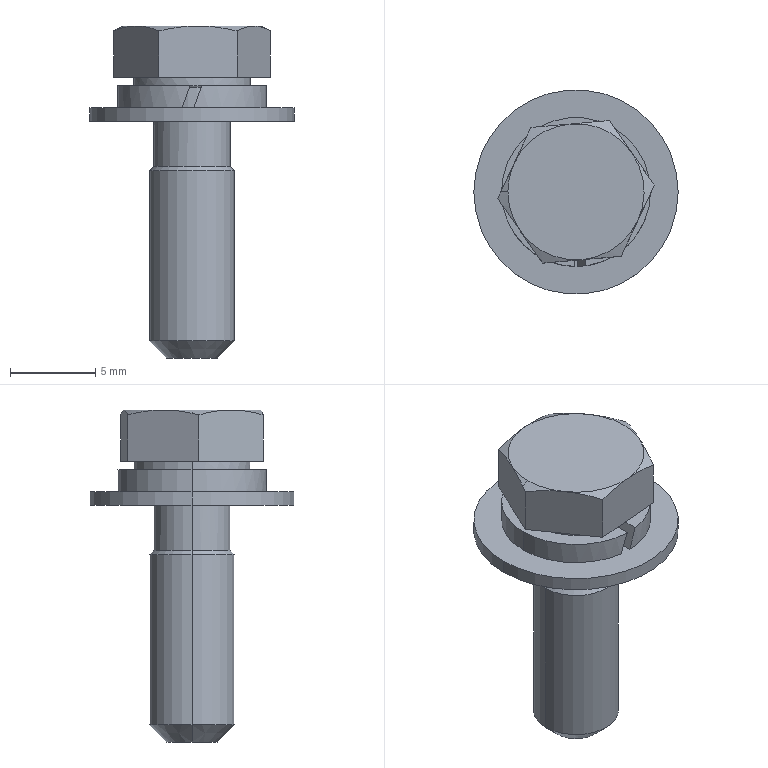Part | NX | features BREP 1 | 1 solid | 41 faces | box 12 x 12 x 19.5 mm | volume 603.235 mm3 | plane 15 | cylinder 13 | cone 11 | torus 2 | commonest cylinder face diameters 8.75 x3 4.5 x2 4.75 x2 5 x2 6.88 x2 12 x2
STEP:
#1=CARTESIAN_POINT('',(-90.692,-391.421,-6.817));
#2=VERTEX_POINT('',#1);
#3=CARTESIAN_POINT('',(-90.417,-392.5,-6.817));
#4=VERTEX_POINT('',#3);
#5=CARTESIAN_POINT('',(-92.667,-392.5,-6.817));
#6=DIRECTION('',(0.,0.,-1.));
#7=DIRECTION('',(-0.8776,-0.4794,0.));
#8=AXIS2_PLACEMENT_3D('',#5,#6,#7);
#9=CIRCLE('',#8,2.25);
#10=EDGE_CURVE('',#2,#4,#9,.T.);
#11=ORIENTED_EDGE('',*,*,#10,.F.);
#12=CARTESIAN_POINT('',(-90.604,-391.373,-6.717));
#13=VERTEX_POINT('',#12);
#14=CARTESIAN_POINT('',(-90.604,-391.373,-6.817));
#15=DIRECTION('',(-0.4794,0.8776,0.));
#16=DIRECTION('',(0.8776,0.4794,0.));
#17=AXIS2_PLACEMENT_3D('',#14,#15,#16);
#18=CIRCLE('',#17,0.1);
#19=EDGE_CURVE('',#13,#2,#18,.F.);
#20=ORIENTED_EDGE('',*,*,#19,.F.);
#21=CARTESIAN_POINT('',(-92.667,-394.85,-6.717));
#22=VERTEX_POINT('',#21);
#23=CARTESIAN_POINT('',(-90.604,-391.373,-6.717));
#24=CARTESIAN_POINT('',(-89.645,-393.129,-6.717));
#25=CARTESIAN_POINT('',(-90.666,-394.85,-6.717));
#26=CARTESIAN_POINT('',(-92.667,-394.85,-6.717));
#27=(BOUNDED_CURVE()B_SPLINE_CURVE(3,(#23,#24,#25,#26),.UNSPECIFIED.,.F.,.F.)B_SPLINE_CURVE_WITH_KNOTS((4,4),(0.,1.),.PIECEWISE_BEZIER_KNOTS.)CURVE()GEOMETRIC_REPRESENTATION_ITEM()RATIONAL_B_SPLINE_CURVE((1.,0.6735,0.6735,1.))REPRESENTATION_ITEM(''));
#28=EDGE_CURVE('',#13,#22,#27,.T.);
#29=ORIENTED_EDGE('',*,*,#28,.T.);
#30=CARTESIAN_POINT('',(-94.729,-393.627,-6.717));
#31=VERTEX_POINT('',#30);
#32=CARTESIAN_POINT('',(-92.667,-394.85,-6.717));
#33=CARTESIAN_POINT('',(-93.548,-394.85,-6.717));
#34=CARTESIAN_POINT('',(-94.306,-394.4,-6.717));
#35=CARTESIAN_POINT('',(-94.729,-393.627,-6.717));
#36=(BOUNDED_CURVE()B_SPLINE_CURVE(3,(#32,#33,#34,#35),.UNSPECIFIED.,.F.,.F.)B_SPLINE_CURVE_WITH_KNOTS((4,4),(0.,1.),.PIECEWISE_BEZIER_KNOTS.)CURVE()GEOMETRIC_REPRESENTATION_ITEM()RATIONAL_B_SPLINE_CURVE((1.,0.9067,0.9067,1.))REPRESENTATION_ITEM(''));
#37=EDGE_CURVE('',#22,#31,#36,.T.);
#38=ORIENTED_EDGE('',*,*,#37,.T.);
#39=CARTESIAN_POINT('',(-94.641,-393.579,-6.817));
#40=VERTEX_POINT('',#39);
#41=CARTESIAN_POINT('',(-94.729,-393.627,-6.817));
#42=DIRECTION('',(0.4794,-0.8776,0.));
#43=DIRECTION('',(-0.8776,-0.4794,0.));
#44=AXIS2_PLACEMENT_3D('',#41,#42,#43);
#45=CIRCLE('',#44,0.1);
#46=EDGE_CURVE('',#31,#40,#45,.F.);
#47=ORIENTED_EDGE('',*,*,#46,.T.);
#48=CARTESIAN_POINT('',(-92.667,-392.5,-6.817));
#49=DIRECTION('',(0.,0.,-1.));
#50=DIRECTION('',(-0.8776,-0.4794,0.));
#51=AXIS2_PLACEMENT_3D('',#48,#49,#50);
#52=CIRCLE('',#51,2.25);
#53=EDGE_CURVE('',#4,#40,#52,.T.);
#54=ORIENTED_EDGE('',*,*,#53,.F.);
#55=EDGE_LOOP('',(#11,#20,#29,#38,#47,#54));
#56=FACE_BOUND('',#55,.T.);
#57=CARTESIAN_POINT('',(-92.667,-392.5,-6.817));
#58=DIRECTION('',(0.,0.,1.));
#59=DIRECTION('',(1.,0.,0.));
#60=AXIS2_PLACEMENT_3D('',#57,#58,#59);
#61=TOROIDAL_SURFACE('',#60,2.35,0.1);
#62=ADVANCED_FACE('',(#56),#61,.F.);
#63=CARTESIAN_POINT('',(-90.292,-392.5,-6.717));
#64=VERTEX_POINT('',#63);
#65=CARTESIAN_POINT('',(-92.084,-394.802,-6.717));
#66=VERTEX_POINT('',#65);
#67=CARTESIAN_POINT('',(-92.667,-392.5,-6.717));
#68=DIRECTION('',(0.,0.,-1.));
#69=DIRECTION('',(-1.,0.,0.));
#70=AXIS2_PLACEMENT_3D('',#67,#68,#69);
#71=CIRCLE('',#70,2.375);
#72=EDGE_CURVE('',#64,#66,#71,.T.);
#73=ORIENTED_EDGE('',*,*,#72,.F.);
#74=CARTESIAN_POINT('',(-90.292,-392.5,-8.817));
#75=VERTEX_POINT('',#74);
#76=CARTESIAN_POINT('',(-90.292,-392.5,-7.367));
#77=DIRECTION('',(0.,0.,-1.));
#78=VECTOR('',#77,1000.);
#79=LINE('',#76,#78);
#80=EDGE_CURVE('',#75,#64,#79,.F.);
#81=ORIENTED_EDGE('',*,*,#80,.F.);
#82=CARTESIAN_POINT('',(-95.042,-392.5,-8.817));
#83=VERTEX_POINT('',#82);
#84=CARTESIAN_POINT('',(-92.667,-392.5,-8.817));
#85=DIRECTION('',(0.,0.,1.));
#86=DIRECTION('',(-1.,0.,0.));
#87=AXIS2_PLACEMENT_3D('',#84,#85,#86);
#88=CIRCLE('',#87,2.375);
#89=EDGE_CURVE('',#83,#75,#88,.T.);
#90=ORIENTED_EDGE('',*,*,#89,.F.);
#91=CARTESIAN_POINT('',(-95.042,-392.5,-6.717));
#92=VERTEX_POINT('',#91);
#93=CARTESIAN_POINT('',(-95.042,-392.5,-7.367));
#94=DIRECTION('',(0.,0.,-1.));
#95=VECTOR('',#94,1000.);
#96=LINE('',#93,#95);
#97=EDGE_CURVE('',#83,#92,#96,.F.);
#98=ORIENTED_EDGE('',*,*,#97,.T.);
#99=CARTESIAN_POINT('',(-92.776,-394.872,-6.717));
#100=VERTEX_POINT('',#99);
#101=CARTESIAN_POINT('',(-92.667,-392.5,-6.717));
#102=DIRECTION('',(0.,0.,-1.));
#103=DIRECTION('',(-1.,0.,0.));
#104=AXIS2_PLACEMENT_3D('',#101,#102,#103);
#105=CIRCLE('',#104,2.375);
#106=EDGE_CURVE('',#100,#92,#105,.T.);
#107=ORIENTED_EDGE('',*,*,#106,.F.);
#108=CARTESIAN_POINT('',(-93.249,-394.802,-8.017));
#109=VERTEX_POINT('',#108);
#110=CARTESIAN_POINT('',(-93.249,-394.802,-8.017));
#111=CARTESIAN_POINT('',(-93.094,-394.842,-7.591));
#112=CARTESIAN_POINT('',(-92.936,-394.865,-7.156));
#113=CARTESIAN_POINT('',(-92.776,-394.872,-6.717));
#114=(BOUNDED_CURVE()B_SPLINE_CURVE(3,(#110,#111,#112,#113),.UNSPECIFIED.,.F.,.F.)B_SPLINE_CURVE_WITH_KNOTS((4,4),(0.,1.),.PIECEWISE_BEZIER_KNOTS.)CURVE()GEOMETRIC_REPRESENTATION_ITEM()RATIONAL_B_SPLINE_CURVE((1.,0.9966,0.9966,1.))REPRESENTATION_ITEM(''));
#115=EDGE_CURVE('',#109,#100,#114,.T.);
#116=ORIENTED_EDGE('',*,*,#115,.F.);
#117=CARTESIAN_POINT('',(-92.557,-394.872,-8.017));
#118=VERTEX_POINT('',#117);
#119=CARTESIAN_POINT('',(-92.667,-392.5,-8.017));
#120=DIRECTION('',(0.,0.,1.));
#121=DIRECTION('',(-1.,0.,0.));
#122=AXIS2_PLACEMENT_3D('',#119,#120,#121);
#123=CIRCLE('',#122,2.375);
#124=EDGE_CURVE('',#109,#118,#123,.T.);
#125=ORIENTED_EDGE('',*,*,#124,.T.);
#126=CARTESIAN_POINT('',(-92.084,-394.802,-6.717));
#127=CARTESIAN_POINT('',(-92.239,-394.842,-7.143));
#128=CARTESIAN_POINT('',(-92.398,-394.865,-7.578));
#129=CARTESIAN_POINT('',(-92.557,-394.872,-8.017));
#130=(BOUNDED_CURVE()B_SPLINE_CURVE(3,(#126,#127,#128,#129),.UNSPECIFIED.,.F.,.F.)B_SPLINE_CURVE_WITH_KNOTS((4,4),(0.,1.),.PIECEWISE_BEZIER_KNOTS.)CURVE()GEOMETRIC_REPRESENTATION_ITEM()RATIONAL_B_SPLINE_CURVE((1.,0.9966,0.9966,1.))REPRESENTATION_ITEM(''));
#131=EDGE_CURVE('',#66,#118,#130,.T.);
#132=ORIENTED_EDGE('',*,*,#131,.F.);
#133=EDGE_LOOP('',(#73,#81,#90,#98,#107,#116,#125,#132));
#134=FACE_BOUND('',#133,.T.);
#135=CARTESIAN_POINT('',(-92.667,-392.5,-7.367));
#136=DIRECTION('',(0.,0.,-1.));
#137=DIRECTION('',(1.,0.,0.));
#138=AXIS2_PLACEMENT_3D('',#135,#136,#137);
#139=CYLINDRICAL_SURFACE('',#138,2.375);
#140=ADVANCED_FACE('',(#134),#139,.F.);
#141=CARTESIAN_POINT('',(-98.667,-392.5,-8.017));
#142=VERTEX_POINT('',#141);
#143=CARTESIAN_POINT('',(-86.667,-392.5,-8.017));
#144=VERTEX_POINT('',#143);
#145=CARTESIAN_POINT('',(-92.667,-392.5,-8.017));
#146=DIRECTION('',(0.,0.,-1.));
#147=DIRECTION('',(-1.,0.,0.));
#148=AXIS2_PLACEMENT_3D('',#145,#146,#147);
#149=CIRCLE('',#148,6.);
#150=EDGE_CURVE('',#142,#144,#149,.T.);
#151=ORIENTED_EDGE('',*,*,#150,.T.);
#152=CARTESIAN_POINT('',(-86.667,-392.5,-8.817));
#153=VERTEX_POINT('',#152);
#154=CARTESIAN_POINT('',(-86.667,-392.5,-8.517));
#155=DIRECTION('',(0.,0.,-1.));
#156=VECTOR('',#155,1000.);
#157=LINE('',#154,#156);
#158=EDGE_CURVE('',#153,#144,#157,.F.);
#159=ORIENTED_EDGE('',*,*,#158,.F.);
#160=CARTESIAN_POINT('',(-98.667,-392.5,-8.817));
#161=VERTEX_POINT('',#160);
#162=CARTESIAN_POINT('',(-92.667,-392.5,-8.817));
#163=DIRECTION('',(0.,0.,-1.));
#164=DIRECTION('',(-1.,0.,0.));
#165=AXIS2_PLACEMENT_3D('',#162,#163,#164);
#166=CIRCLE('',#165,6.);
#167=EDGE_CURVE('',#161,#153,#166,.T.);
#168=ORIENTED_EDGE('',*,*,#167,.F.);
#169=CARTESIAN_POINT('',(-98.667,-392.5,-8.517));
#170=DIRECTION('',(0.,0.,-1.));
#171=VECTOR('',#170,1000.);
#172=LINE('',#169,#171);
#173=EDGE_CURVE('',#161,#142,#172,.F.);
#174=ORIENTED_EDGE('',*,*,#173,.T.);
#175=EDGE_LOOP('',(#151,#159,#168,#174));
#176=FACE_BOUND('',#175,.T.);
#177=CARTESIAN_POINT('',(-92.667,-392.5,-8.517));
#178=DIRECTION('',(0.,0.,-1.));
#179=DIRECTION('',(1.,0.,0.));
#180=AXIS2_PLACEMENT_3D('',#177,#178,#179);
#181=CYLINDRICAL_SURFACE('',#180,6.);
#182=ADVANCED_FACE('',(#176),#181,.T.);
#183=CARTESIAN_POINT('',(-97.042,-392.5,-6.717));
#184=VERTEX_POINT('',#183);
#185=CARTESIAN_POINT('',(-88.292,-392.5,-6.717));
#186=VERTEX_POINT('',#185);
#187=CARTESIAN_POINT('',(-92.667,-392.5,-6.717));
#188=DIRECTION('',(0.,0.,-1.));
#189=DIRECTION('',(-1.,0.,0.));
#190=AXIS2_PLACEMENT_3D('',#187,#188,#189);
#191=CIRCLE('',#190,4.375);
#192=EDGE_CURVE('',#184,#186,#191,.T.);
#193=ORIENTED_EDGE('',*,*,#192,.T.);
#194=CARTESIAN_POINT('',(-88.292,-392.5,-8.017));
#195=VERTEX_POINT('',#194);
#196=CARTESIAN_POINT('',(-88.292,-392.5,-7.367));
#197=DIRECTION('',(0.,0.,-1.));
#198=VECTOR('',#197,1000.);
#199=LINE('',#196,#198);
#200=EDGE_CURVE('',#186,#195,#199,.T.);
#201=ORIENTED_EDGE('',*,*,#200,.T.);
#202=CARTESIAN_POINT('',(-97.042,-392.5,-8.017));
#203=VERTEX_POINT('',#202);
#204=CARTESIAN_POINT('',(-92.667,-392.5,-8.017));
#205=DIRECTION('',(0.,0.,1.));
#206=DIRECTION('',(-1.,0.,0.));
#207=AXIS2_PLACEMENT_3D('',#204,#205,#206);
#208=CIRCLE('',#207,4.375);
#209=EDGE_CURVE('',#195,#203,#208,.T.);
#210=ORIENTED_EDGE('',*,*,#209,.T.);
#211=CARTESIAN_POINT('',(-97.042,-392.5,-7.367));
#212=DIRECTION('',(0.,0.,-1.));
#213=VECTOR('',#212,1000.);
#214=LINE('',#211,#213);
#215=EDGE_CURVE('',#184,#203,#214,.T.);
#216=ORIENTED_EDGE('',*,*,#215,.F.);
#217=EDGE_LOOP('',(#193,#201,#210,#216));
#218=FACE_BOUND('',#217,.T.);
#219=CARTESIAN_POINT('',(-92.667,-392.5,-7.367));
#220=DIRECTION('',(0.,0.,-1.));
#221=DIRECTION('',(1.,0.,0.));
#222=AXIS2_PLACEMENT_3D('',#219,#220,#221);
#223=CYLINDRICAL_SURFACE('',#222,4.375);
#224=ADVANCED_FACE('',(#218),#223,.T.);
#225=CARTESIAN_POINT('',(-92.776,-396.874,-6.717));
#226=VERTEX_POINT('',#225);
#227=CARTESIAN_POINT('',(-92.667,-392.5,-6.717));
#228=DIRECTION('',(0.,0.,-1.));
#229=DIRECTION('',(-1.,0.,0.));
#230=AXIS2_PLACEMENT_3D('',#227,#228,#229);
#231=CIRCLE('',#230,4.375);
#232=EDGE_CURVE('',#226,#184,#231,.T.);
#233=ORIENTED_EDGE('',*,*,#232,.T.);
#234=ORIENTED_EDGE('',*,*,#215,.T.);
#235=CARTESIAN_POINT('',(-93.249,-396.836,-8.017));
#236=VERTEX_POINT('',#235);
#237=CARTESIAN_POINT('',(-92.667,-392.5,-8.017));
#238=DIRECTION('',(0.,0.,1.));
#239=DIRECTION('',(-1.,0.,0.));
#240=AXIS2_PLACEMENT_3D('',#237,#238,#239);
#241=CIRCLE('',#240,4.375);
#242=EDGE_CURVE('',#203,#236,#241,.T.);
#243=ORIENTED_EDGE('',*,*,#242,.T.);
#244=CARTESIAN_POINT('',(-93.249,-396.836,-8.017));
#245=CARTESIAN_POINT('',(-93.092,-396.857,-7.585));
#246=CARTESIAN_POINT('',(-92.934,-396.87,-7.152));
#247=CARTESIAN_POINT('',(-92.776,-396.874,-6.717));
#248=(BOUNDED_CURVE()B_SPLINE_CURVE(3,(#244,#245,#246,#247),.UNSPECIFIED.,.F.,.F.)B_SPLINE_CURVE_WITH_KNOTS((4,4),(0.,1.),.PIECEWISE_BEZIER_KNOTS.)CURVE()GEOMETRIC_REPRESENTATION_ITEM()RATIONAL_B_SPLINE_CURVE((1.,0.999,0.999,1.))REPRESENTATION_ITEM(''));
#249=EDGE_CURVE('',#236,#226,#248,.T.);
#250=ORIENTED_EDGE('',*,*,#249,.T.);
#251=EDGE_LOOP('',(#233,#234,#243,#250));
#252=FACE_BOUND('',#251,.T.);
#253=CARTESIAN_POINT('',(-92.667,-392.5,-7.367));
#254=DIRECTION('',(0.,0.,-1.));
#255=DIRECTION('',(1.,0.,0.));
#256=AXIS2_PLACEMENT_3D('',#253,#254,#255);
#257=CYLINDRICAL_SURFACE('',#256,4.375);
#258=ADVANCED_FACE('',(#252),#257,.T.);
#259=CARTESIAN_POINT('',(-90.417,-392.5,-11.468));
#260=VERTEX_POINT('',#259);
#261=CARTESIAN_POINT('',(-94.917,-392.5,-11.468));
#262=VERTEX_POINT('',#261);
#263=CARTESIAN_POINT('',(-92.667,-392.5,-11.468));
#264=DIRECTION('',(0.,0.,1.));
#265=DIRECTION('',(1.,0.,0.));
#266=AXIS2_PLACEMENT_3D('',#263,#264,#265);
#267=CIRCLE('',#266,2.25);
#268=EDGE_CURVE('',#260,#262,#267,.T.);
#269=ORIENTED_EDGE('',*,*,#268,.T.);
#270=CARTESIAN_POINT('',(-94.917,-392.5,-6.817));
#271=VERTEX_POINT('',#270);
#272=CARTESIAN_POINT('',(-94.917,-392.5,-12.967));
#273=DIRECTION('',(0.,0.,1.));
#274=VECTOR('',#273,1000.);
#275=LINE('',#272,#274);
#276=EDGE_CURVE('',#262,#271,#275,.T.);
#277=ORIENTED_EDGE('',*,*,#276,.T.);
#278=CARTESIAN_POINT('',(-92.667,-392.5,-6.817));
#279=DIRECTION('',(0.,0.,-1.));
#280=DIRECTION('',(-0.8776,-0.4794,0.));
#281=AXIS2_PLACEMENT_3D('',#278,#279,#280);
#282=CIRCLE('',#281,2.25);
#283=EDGE_CURVE('',#271,#2,#282,.T.);
#284=ORIENTED_EDGE('',*,*,#283,.T.);
#285=ORIENTED_EDGE('',*,*,#10,.T.);
#286=CARTESIAN_POINT('',(-90.417,-392.5,-12.967));
#287=DIRECTION('',(0.,0.,1.));
#288=VECTOR('',#287,1000.);
#289=LINE('',#286,#288);
#290=EDGE_CURVE('',#260,#4,#289,.T.);
#291=ORIENTED_EDGE('',*,*,#290,.F.);
#292=EDGE_LOOP('',(#269,#277,#284,#285,#291));
#293=FACE_BOUND('',#292,.T.);
#294=CARTESIAN_POINT('',(-92.667,-392.5,-12.967));
#295=DIRECTION('',(0.,0.,1.));
#296=DIRECTION('',(-1.,0.,0.));
#297=AXIS2_PLACEMENT_3D('',#294,#295,#296);
#298=CYLINDRICAL_SURFACE('',#297,2.25);
#299=ADVANCED_FACE('',(#293),#298,.T.);
#300=ORIENTED_EDGE('',*,*,#268,.F.);
#301=CARTESIAN_POINT('',(-90.167,-392.5,-11.718));
#302=VERTEX_POINT('',#301);
#303=CARTESIAN_POINT('',(-90.167,-392.5,-11.718));
#304=DIRECTION('',(0.7071,0.,-0.7071));
#305=VECTOR('',#304,1000.);
#306=LINE('',#303,#305);
#307=EDGE_CURVE('',#302,#260,#306,.F.);
#308=ORIENTED_EDGE('',*,*,#307,.F.);
#309=CARTESIAN_POINT('',(-95.167,-392.5,-11.718));
#310=VERTEX_POINT('',#309);
#311=CARTESIAN_POINT('',(-92.667,-392.5,-11.718));
#312=DIRECTION('',(0.,0.,1.));
#313=DIRECTION('',(0.8776,0.4794,0.));
#314=AXIS2_PLACEMENT_3D('',#311,#312,#313);
#315=CIRCLE('',#314,2.5);
#316=EDGE_CURVE('',#302,#310,#315,.T.);
#317=ORIENTED_EDGE('',*,*,#316,.T.);
#318=CARTESIAN_POINT('',(-95.167,-392.5,-11.718));
#319=DIRECTION('',(-0.7071,0.,-0.7071));
#320=VECTOR('',#319,1000.);
#321=LINE('',#318,#320);
#322=EDGE_CURVE('',#310,#262,#321,.F.);
#323=ORIENTED_EDGE('',*,*,#322,.T.);
#324=EDGE_LOOP('',(#300,#308,#317,#323));
#325=FACE_BOUND('',#324,.T.);
#326=CARTESIAN_POINT('',(-92.667,-392.5,-11.718));
#327=DIRECTION('',(0.,0.,-1.));
#328=DIRECTION('',(1.,0.,0.));
#329=AXIS2_PLACEMENT_3D('',#326,#327,#328);
#330=CONICAL_SURFACE('',#329,2.5,0.7854);
#331=ADVANCED_FACE('',(#325),#330,.T.);
#332=CARTESIAN_POINT('',(-96.107,-392.5,-6.717));
#333=VERTEX_POINT('',#332);
#334=CARTESIAN_POINT('',(-89.227,-392.5,-6.717));
#335=VERTEX_POINT('',#334);
#336=CARTESIAN_POINT('',(-92.667,-392.5,-6.717));
#337=DIRECTION('',(0.,0.,-1.));
#338=DIRECTION('',(1.,0.,0.));
#339=AXIS2_PLACEMENT_3D('',#336,#337,#338);
#340=CIRCLE('',#339,3.44);
#341=EDGE_CURVE('',#333,#335,#340,.T.);
#342=ORIENTED_EDGE('',*,*,#341,.F.);
#343=CARTESIAN_POINT('',(-96.107,-392.5,-6.217));
#344=VERTEX_POINT('',#343);
#345=CARTESIAN_POINT('',(-96.107,-392.5,-12.967));
#346=DIRECTION('',(0.,0.,1.));
#347=VECTOR('',#346,1000.);
#348=LINE('',#345,#347);
#349=EDGE_CURVE('',#333,#344,#348,.T.);
#350=ORIENTED_EDGE('',*,*,#349,.T.);
#351=CARTESIAN_POINT('',(-89.227,-392.5,-6.217));
#352=VERTEX_POINT('',#351);
#353=CARTESIAN_POINT('',(-92.667,-392.5,-6.217));
#354=DIRECTION('',(0.,0.,-1.));
#355=DIRECTION('',(1.,0.,0.));
#356=AXIS2_PLACEMENT_3D('',#353,#354,#355);
#357=CIRCLE('',#356,3.44);
#358=EDGE_CURVE('',#344,#352,#357,.T.);
#359=ORIENTED_EDGE('',*,*,#358,.T.);
#360=CARTESIAN_POINT('',(-89.227,-392.5,-12.967));
#361=DIRECTION('',(0.,0.,1.));
#362=VECTOR('',#361,1000.);
#363=LINE('',#360,#362);
#364=EDGE_CURVE('',#335,#352,#363,.T.);
#365=ORIENTED_EDGE('',*,*,#364,.F.);
#366=EDGE_LOOP('',(#342,#350,#359,#365));
#367=FACE_BOUND('',#366,.T.);
#368=CARTESIAN_POINT('',(-92.667,-392.5,-12.967));
#369=DIRECTION('',(0.,0.,1.));
#370=DIRECTION('',(-1.,0.,0.));
#371=AXIS2_PLACEMENT_3D('',#368,#369,#370);
#372=CYLINDRICAL_SURFACE('',#371,3.44);
#373=ADVANCED_FACE('',(#367),#372,.T.);
#374=CARTESIAN_POINT('',(-90.167,-392.5,-21.717));
#375=VERTEX_POINT('',#374);
#376=CARTESIAN_POINT('',(-95.167,-392.5,-21.717));
#377=VERTEX_POINT('',#376);
#378=CARTESIAN_POINT('',(-92.667,-392.5,-21.717));
#379=DIRECTION('',(0.,0.,1.));
#380=DIRECTION('',(1.,0.,0.));
#381=AXIS2_PLACEMENT_3D('',#378,#379,#380);
#382=CIRCLE('',#381,2.5);
#383=EDGE_CURVE('',#375,#377,#382,.T.);
#384=ORIENTED_EDGE('',*,*,#383,.T.);
#385=CARTESIAN_POINT('',(-95.167,-392.5,-12.967));
#386=DIRECTION('',(0.,0.,1.));
#387=VECTOR('',#386,1000.);
#388=LINE('',#385,#387);
#389=EDGE_CURVE('',#377,#310,#388,.T.);
#390=ORIENTED_EDGE('',*,*,#389,.T.);
#391=ORIENTED_EDGE('',*,*,#316,.F.);
#392=CARTESIAN_POINT('',(-90.167,-392.5,-12.967));
#393=DIRECTION('',(0.,0.,1.));
#394=VECTOR('',#393,1000.);
#395=LINE('',#392,#394);
#396=EDGE_CURVE('',#375,#302,#395,.T.);
#397=ORIENTED_EDGE('',*,*,#396,.F.);
#398=EDGE_LOOP('',(#384,#390,#391,#397));
#399=FACE_BOUND('',#398,.T.);
#400=CARTESIAN_POINT('',(-92.667,-392.5,-12.967));
#401=DIRECTION('',(0.,0.,1.));
#402=DIRECTION('',(-1.,0.,0.));
#403=AXIS2_PLACEMENT_3D('',#400,#401,#402);
#404=CYLINDRICAL_SURFACE('',#403,2.5);
#405=ADVANCED_FACE('',(#399),#404,.T.);
#406=CARTESIAN_POINT('',(-91.167,-392.5,-22.717));
#407=VERTEX_POINT('',#406);
#408=CARTESIAN_POINT('',(-94.167,-392.5,-22.717));
#409=VERTEX_POINT('',#408);
#410=CARTESIAN_POINT('',(-92.667,-392.5,-22.717));
#411=DIRECTION('',(0.,0.,1.));
#412=DIRECTION('',(1.,0.,0.));
#413=AXIS2_PLACEMENT_3D('',#410,#411,#412);
#414=CIRCLE('',#413,1.5);
#415=EDGE_CURVE('',#407,#409,#414,.T.);
#416=ORIENTED_EDGE('',*,*,#415,.T.);
#417=CARTESIAN_POINT('',(-95.167,-392.5,-21.717));
#418=DIRECTION('',(-0.7071,0.,0.7071));
#419=VECTOR('',#418,1000.);
#420=LINE('',#417,#419);
#421=EDGE_CURVE('',#409,#377,#420,.T.);
#422=ORIENTED_EDGE('',*,*,#421,.T.);
#423=ORIENTED_EDGE('',*,*,#383,.F.);
#424=CARTESIAN_POINT('',(-90.167,-392.5,-21.717));
#425=DIRECTION('',(0.7071,0.,0.7071));
#426=VECTOR('',#425,1000.);
#427=LINE('',#424,#426);
#428=EDGE_CURVE('',#407,#375,#427,.T.);
#429=ORIENTED_EDGE('',*,*,#428,.F.);
#430=EDGE_LOOP('',(#416,#422,#423,#429));
#431=FACE_BOUND('',#430,.T.);
#432=CARTESIAN_POINT('',(-92.667,-392.5,-21.717));
#433=DIRECTION('',(0.,0.,1.));
#434=DIRECTION('',(-1.,0.,0.));
#435=AXIS2_PLACEMENT_3D('',#432,#433,#434);
#436=CONICAL_SURFACE('',#435,2.5,0.7854);
#437=ADVANCED_FACE('',(#431),#436,.T.);
#438=CARTESIAN_POINT('',(-95.943,-394.794,-3.217));
#439=VERTEX_POINT('',#438);
#440=CARTESIAN_POINT('',(-96.667,-392.5,-3.217));
#441=VERTEX_POINT('',#440);
#442=CARTESIAN_POINT('',(-92.667,-392.5,-3.217));
#443=DIRECTION('',(0.,0.,-1.));
#444=DIRECTION('',(-1.,0.,0.));
#445=AXIS2_PLACEMENT_3D('',#442,#443,#444);
#446=CIRCLE('',#445,4.);
#447=EDGE_CURVE('',#439,#441,#446,.T.);
#448=ORIENTED_EDGE('',*,*,#447,.T.);
#449=CARTESIAN_POINT('',(-97.08,-392.5,-3.409));
#450=VERTEX_POINT('',#449);
#451=CARTESIAN_POINT('',(-97.289,-392.5,-3.507));
#452=DIRECTION('',(-0.9063,0.,-0.4226));
#453=VECTOR('',#452,1000.);
#454=LINE('',#451,#453);
#455=EDGE_CURVE('',#441,#450,#454,.T.);
#456=ORIENTED_EDGE('',*,*,#455,.T.);
#457=CARTESIAN_POINT('',(-97.268,-392.903,-3.505));
#458=VERTEX_POINT('',#457);
#459=CARTESIAN_POINT('',(-97.08,-392.5,-3.409));
#460=CARTESIAN_POINT('',(-97.142,-392.633,-3.438));
#461=CARTESIAN_POINT('',(-97.204,-392.767,-3.47));
#462=CARTESIAN_POINT('',(-97.268,-392.903,-3.505));
#463=B_SPLINE_CURVE_WITH_KNOTS('',3,(#459,#460,#461,#462),.UNSPECIFIED.,.F.,.F.,(4,4),(0.,1.),.PIECEWISE_BEZIER_KNOTS.);
#464=EDGE_CURVE('',#450,#458,#463,.T.);
#465=ORIENTED_EDGE('',*,*,#464,.T.);
#466=CARTESIAN_POINT('',(-97.268,-392.903,-3.505));
#467=CARTESIAN_POINT('',(-96.832,-393.525,-3.328));
#468=CARTESIAN_POINT('',(-96.392,-394.154,-3.217));
#469=CARTESIAN_POINT('',(-95.943,-394.794,-3.217));
#470=B_SPLINE_CURVE_WITH_KNOTS('',3,(#466,#467,#468,#469),.UNSPECIFIED.,.F.,.F.,(4,4),(0.,0.002327),.UNSPECIFIED.);
#471=EDGE_CURVE('',#458,#439,#470,.T.);
#472=ORIENTED_EDGE('',*,*,#471,.T.);
#473=EDGE_LOOP('',(#448,#456,#465,#472));
#474=FACE_BOUND('',#473,.T.);
#475=CARTESIAN_POINT('',(-92.667,-392.5,-3.507));
#476=DIRECTION('',(0.,0.,-1.));
#477=DIRECTION('',(1.,0.,0.));
#478=AXIS2_PLACEMENT_3D('',#475,#476,#477);
#479=CONICAL_SURFACE('',#478,4.623,1.134);
#480=ADVANCED_FACE('',(#474),#479,.T.);
#481=ORIENTED_EDGE('',*,*,#89,.T.);
#482=CARTESIAN_POINT('',(-92.667,-392.5,-8.817));
#483=DIRECTION('',(0.,0.,1.));
#484=DIRECTION('',(-1.,0.,0.));
#485=AXIS2_PLACEMENT_3D('',#482,#483,#484);
#486=CIRCLE('',#485,2.375);
#487=EDGE_CURVE('',#75,#83,#486,.T.);
#488=ORIENTED_EDGE('',*,*,#487,.T.);
#489=EDGE_LOOP('',(#481,#488));
#490=FACE_BOUND('',#489,.T.);
#491=ORIENTED_EDGE('',*,*,#167,.T.);
#492=CARTESIAN_POINT('',(-92.667,-392.5,-8.817));
#493=DIRECTION('',(0.,0.,-1.));
#494=DIRECTION('',(-1.,0.,0.));
#495=AXIS2_PLACEMENT_3D('',#492,#493,#494);
#496=CIRCLE('',#495,6.);
#497=EDGE_CURVE('',#153,#161,#496,.T.);
#498=ORIENTED_EDGE('',*,*,#497,.T.);
#499=EDGE_LOOP('',(#491,#498));
#500=FACE_BOUND('',#499,.T.);
#501=CARTESIAN_POINT('',(-92.667,-392.5,-8.817));
#502=DIRECTION('',(0.,0.,-1.));
#503=DIRECTION('',(1.,0.,0.));
#504=AXIS2_PLACEMENT_3D('',#501,#502,#503);
#505=PLANE('',#504);
#506=ADVANCED_FACE('',(#490,#500),#505,.T.);
#507=ORIENTED_EDGE('',*,*,#80,.T.);
#508=CARTESIAN_POINT('',(-92.667,-392.5,-6.717));
#509=DIRECTION('',(0.,0.,-1.));
#510=DIRECTION('',(-1.,0.,0.));
#511=AXIS2_PLACEMENT_3D('',#508,#509,#510);
#512=CIRCLE('',#511,2.375);
#513=EDGE_CURVE('',#92,#64,#512,.T.);
#514=ORIENTED_EDGE('',*,*,#513,.F.);
#515=ORIENTED_EDGE('',*,*,#97,.F.);
#516=ORIENTED_EDGE('',*,*,#487,.F.);
#517=EDGE_LOOP('',(#507,#514,#515,#516));
#518=FACE_BOUND('',#517,.T.);
#519=CARTESIAN_POINT('',(-92.667,-392.5,-7.367));
#520=DIRECTION('',(0.,0.,-1.));
#521=DIRECTION('',(1.,0.,0.));
#522=AXIS2_PLACEMENT_3D('',#519,#520,#521);
#523=CYLINDRICAL_SURFACE('',#522,2.375);
#524=ADVANCED_FACE('',(#518),#523,.F.);
#525=ORIENTED_EDGE('',*,*,#158,.T.);
#526=CARTESIAN_POINT('',(-92.667,-392.5,-8.017));
#527=DIRECTION('',(0.,0.,-1.));
#528=DIRECTION('',(-1.,0.,0.));
#529=AXIS2_PLACEMENT_3D('',#526,#527,#528);
#530=CIRCLE('',#529,6.);
#531=EDGE_CURVE('',#144,#142,#530,.T.);
#532=ORIENTED_EDGE('',*,*,#531,.T.);
#533=ORIENTED_EDGE('',*,*,#173,.F.);
#534=ORIENTED_EDGE('',*,*,#497,.F.);
#535=EDGE_LOOP('',(#525,#532,#533,#534));
#536=FACE_BOUND('',#535,.T.);
#537=CARTESIAN_POINT('',(-92.667,-392.5,-8.517));
#538=DIRECTION('',(0.,0.,-1.));
#539=DIRECTION('',(1.,0.,0.));
#540=AXIS2_PLACEMENT_3D('',#537,#538,#539);
#541=CYLINDRICAL_SURFACE('',#540,6.);
#542=ADVANCED_FACE('',(#536),#541,.T.);
#543=ORIENTED_EDGE('',*,*,#28,.F.);
#544=CARTESIAN_POINT('',(-92.667,-390.15,-6.717));
#545=VERTEX_POINT('',#544);
#546=CARTESIAN_POINT('',(-92.667,-390.15,-6.717));
#547=CARTESIAN_POINT('',(-91.785,-390.15,-6.717));
#548=CARTESIAN_POINT('',(-91.027,-390.6,-6.717));
#549=CARTESIAN_POINT('',(-90.604,-391.373,-6.717));
#550=(BOUNDED_CURVE()B_SPLINE_CURVE(3,(#546,#547,#548,#549),.UNSPECIFIED.,.F.,.F.)B_SPLINE_CURVE_WITH_KNOTS((4,4),(0.,1.),.PIECEWISE_BEZIER_KNOTS.)CURVE()GEOMETRIC_REPRESENTATION_ITEM()RATIONAL_B_SPLINE_CURVE((1.,0.9067,0.9067,1.))REPRESENTATION_ITEM(''));
#551=EDGE_CURVE('',#545,#13,#550,.T.);
#552=ORIENTED_EDGE('',*,*,#551,.F.);
#553=CARTESIAN_POINT('',(-94.729,-393.627,-6.717));
#554=CARTESIAN_POINT('',(-95.688,-391.871,-6.717));
#555=CARTESIAN_POINT('',(-94.667,-390.15,-6.717));
#556=CARTESIAN_POINT('',(-92.667,-390.15,-6.717));
#557=(BOUNDED_CURVE()B_SPLINE_CURVE(3,(#553,#554,#555,#556),.UNSPECIFIED.,.F.,.F.)B_SPLINE_CURVE_WITH_KNOTS((4,4),(0.,1.),.PIECEWISE_BEZIER_KNOTS.)CURVE()GEOMETRIC_REPRESENTATION_ITEM()RATIONAL_B_SPLINE_CURVE((1.,0.6735,0.6735,1.))REPRESENTATION_ITEM(''));
#558=EDGE_CURVE('',#31,#545,#557,.T.);
#559=ORIENTED_EDGE('',*,*,#558,.F.);
#560=ORIENTED_EDGE('',*,*,#37,.F.);
#561=EDGE_LOOP('',(#543,#552,#559,#560));
#562=FACE_BOUND('',#561,.T.);
#563=ORIENTED_EDGE('',*,*,#106,.T.);
#564=ORIENTED_EDGE('',*,*,#513,.T.);
#565=ORIENTED_EDGE('',*,*,#72,.T.);
#566=CARTESIAN_POINT('',(-92.084,-395.89,-6.717));
#567=VERTEX_POINT('',#566);
#568=CARTESIAN_POINT('',(-92.084,-392.5,-6.717));
#569=DIRECTION('',(0.,1.,0.));
#570=VECTOR('',#569,1000.);
#571=LINE('',#568,#570);
#572=EDGE_CURVE('',#567,#66,#571,.T.);
#573=ORIENTED_EDGE('',*,*,#572,.F.);
#574=CARTESIAN_POINT('',(-92.776,-395.938,-6.717));
#575=VERTEX_POINT('',#574);
#576=CARTESIAN_POINT('',(-92.667,-392.5,-6.717));
#577=DIRECTION('',(0.,0.,1.));
#578=DIRECTION('',(1.,0.,0.));
#579=AXIS2_PLACEMENT_3D('',#576,#577,#578);
#580=CIRCLE('',#579,3.44);
#581=EDGE_CURVE('',#575,#567,#580,.T.);
#582=ORIENTED_EDGE('',*,*,#581,.F.);
#583=CARTESIAN_POINT('',(-92.776,-392.5,-6.717));
#584=DIRECTION('',(0.,-1.,0.));
#585=VECTOR('',#584,1000.);
#586=LINE('',#583,#585);
#587=EDGE_CURVE('',#100,#575,#586,.T.);
#588=ORIENTED_EDGE('',*,*,#587,.F.);
#589=EDGE_LOOP('',(#563,#564,#565,#573,#582,#588));
#590=FACE_BOUND('',#589,.T.);
#591=CARTESIAN_POINT('',(-96.107,-392.5,-6.717));
#592=DIRECTION('',(0.,0.,1.));
#593=DIRECTION('',(-1.,0.,0.));
#594=AXIS2_PLACEMENT_3D('',#591,#592,#593);
#595=PLANE('',#594);
#596=ADVANCED_FACE('',(#562,#590),#595,.F.);
#597=ORIENTED_EDGE('',*,*,#249,.F.);
#598=CARTESIAN_POINT('',(-93.249,-392.5,-8.017));
#599=DIRECTION('',(0.,-1.,0.));
#600=VECTOR('',#599,1000.);
#601=LINE('',#598,#600);
#602=EDGE_CURVE('',#109,#236,#601,.T.);
#603=ORIENTED_EDGE('',*,*,#602,.F.);
#604=ORIENTED_EDGE('',*,*,#115,.T.);
#605=ORIENTED_EDGE('',*,*,#587,.T.);
#606=CARTESIAN_POINT('',(-92.776,-392.5,-6.717));
#607=DIRECTION('',(0.,1.,0.));
#608=VECTOR('',#607,1000.);
#609=LINE('',#606,#608);
#610=EDGE_CURVE('',#226,#575,#609,.T.);
#611=ORIENTED_EDGE('',*,*,#610,.F.);
#612=EDGE_LOOP('',(#597,#603,#604,#605,#611));
#613=FACE_BOUND('',#612,.T.);
#614=CARTESIAN_POINT('',(-92.776,-392.5,-6.717));
#615=DIRECTION('',(-0.9397,0.,0.342));
#616=DIRECTION('',(-0.342,0.,-0.9397));
#617=AXIS2_PLACEMENT_3D('',#614,#615,#616);
#618=PLANE('',#617);
#619=ADVANCED_FACE('',(#613),#618,.F.);
#620=ORIENTED_EDGE('',*,*,#124,.F.);
#621=ORIENTED_EDGE('',*,*,#602,.T.);
#622=ORIENTED_EDGE('',*,*,#242,.F.);
#623=ORIENTED_EDGE('',*,*,#209,.F.);
#624=CARTESIAN_POINT('',(-92.557,-396.874,-8.017));
#625=VERTEX_POINT('',#624);
#626=CARTESIAN_POINT('',(-92.667,-392.5,-8.017));
#627=DIRECTION('',(0.,0.,1.));
#628=DIRECTION('',(-1.,0.,0.));
#629=AXIS2_PLACEMENT_3D('',#626,#627,#628);
#630=CIRCLE('',#629,4.375);
#631=EDGE_CURVE('',#625,#195,#630,.T.);
#632=ORIENTED_EDGE('',*,*,#631,.F.);
#633=CARTESIAN_POINT('',(-92.557,-392.5,-8.017));
#634=DIRECTION('',(0.,-1.,0.));
#635=VECTOR('',#634,1000.);
#636=LINE('',#633,#635);
#637=EDGE_CURVE('',#118,#625,#636,.T.);
#638=ORIENTED_EDGE('',*,*,#637,.F.);
#639=EDGE_LOOP('',(#620,#621,#622,#623,#632,#638));
#640=FACE_BOUND('',#639,.T.);
#641=ORIENTED_EDGE('',*,*,#150,.F.);
#642=ORIENTED_EDGE('',*,*,#531,.F.);
#643=EDGE_LOOP('',(#641,#642));
#644=FACE_BOUND('',#643,.T.);
#645=CARTESIAN_POINT('',(-92.667,-392.5,-8.017));
#646=DIRECTION('',(0.,0.,-1.));
#647=DIRECTION('',(1.,0.,0.));
#648=AXIS2_PLACEMENT_3D('',#645,#646,#647);
#649=PLANE('',#648);
#650=ADVANCED_FACE('',(#640,#644),#649,.F.);
#651=ORIENTED_EDGE('',*,*,#19,.T.);
#652=ORIENTED_EDGE('',*,*,#283,.F.);
#653=CARTESIAN_POINT('',(-92.667,-392.5,-6.817));
#654=DIRECTION('',(0.,0.,-1.));
#655=DIRECTION('',(-0.8776,-0.4794,0.));
#656=AXIS2_PLACEMENT_3D('',#653,#654,#655);
#657=CIRCLE('',#656,2.25);
#658=EDGE_CURVE('',#40,#271,#657,.T.);
#659=ORIENTED_EDGE('',*,*,#658,.F.);
#660=ORIENTED_EDGE('',*,*,#46,.F.);
#661=ORIENTED_EDGE('',*,*,#558,.T.);
#662=ORIENTED_EDGE('',*,*,#551,.T.);
#663=EDGE_LOOP('',(#651,#652,#659,#660,#661,#662));
#664=FACE_BOUND('',#663,.T.);
#665=CARTESIAN_POINT('',(-92.667,-392.5,-6.817));
#666=DIRECTION('',(0.,0.,1.));
#667=DIRECTION('',(1.,0.,0.));
#668=AXIS2_PLACEMENT_3D('',#665,#666,#667);
#669=TOROIDAL_SURFACE('',#668,2.35,0.1);
#670=ADVANCED_FACE('',(#664),#669,.F.);
#671=ORIENTED_EDGE('',*,*,#200,.F.);
#672=CARTESIAN_POINT('',(-92.084,-396.836,-6.717));
#673=VERTEX_POINT('',#672);
#674=CARTESIAN_POINT('',(-92.667,-392.5,-6.717));
#675=DIRECTION('',(0.,0.,-1.));
#676=DIRECTION('',(-1.,0.,0.));
#677=AXIS2_PLACEMENT_3D('',#674,#675,#676);
#678=CIRCLE('',#677,4.375);
#679=EDGE_CURVE('',#186,#673,#678,.T.);
#680=ORIENTED_EDGE('',*,*,#679,.T.);
#681=CARTESIAN_POINT('',(-92.084,-396.836,-6.717));
#682=CARTESIAN_POINT('',(-92.241,-396.857,-7.148));
#683=CARTESIAN_POINT('',(-92.399,-396.87,-7.582));
#684=CARTESIAN_POINT('',(-92.557,-396.874,-8.017));
#685=(BOUNDED_CURVE()B_SPLINE_CURVE(3,(#681,#682,#683,#684),.UNSPECIFIED.,.F.,.F.)B_SPLINE_CURVE_WITH_KNOTS((4,4),(0.,1.),.PIECEWISE_BEZIER_KNOTS.)CURVE()GEOMETRIC_REPRESENTATION_ITEM()RATIONAL_B_SPLINE_CURVE((1.,0.999,0.999,1.))REPRESENTATION_ITEM(''));
#686=EDGE_CURVE('',#673,#625,#685,.T.);
#687=ORIENTED_EDGE('',*,*,#686,.T.);
#688=ORIENTED_EDGE('',*,*,#631,.T.);
#689=EDGE_LOOP('',(#671,#680,#687,#688));
#690=FACE_BOUND('',#689,.T.);
#691=CARTESIAN_POINT('',(-92.667,-392.5,-7.367));
#692=DIRECTION('',(0.,0.,-1.));
#693=DIRECTION('',(1.,0.,0.));
#694=AXIS2_PLACEMENT_3D('',#691,#692,#693);
#695=CYLINDRICAL_SURFACE('',#694,4.375);
#696=ADVANCED_FACE('',(#690),#695,.T.);
#697=ORIENTED_EDGE('',*,*,#572,.T.);
#698=ORIENTED_EDGE('',*,*,#131,.T.);
#699=ORIENTED_EDGE('',*,*,#637,.T.);
#700=ORIENTED_EDGE('',*,*,#686,.F.);
#701=CARTESIAN_POINT('',(-92.084,-392.5,-6.717));
#702=DIRECTION('',(0.,1.,0.));
#703=VECTOR('',#702,1000.);
#704=LINE('',#701,#703);
#705=EDGE_CURVE('',#673,#567,#704,.T.);
#706=ORIENTED_EDGE('',*,*,#705,.T.);
#707=EDGE_LOOP('',(#697,#698,#699,#700,#706));
#708=FACE_BOUND('',#707,.T.);
#709=CARTESIAN_POINT('',(-92.084,-392.5,-6.717));
#710=DIRECTION('',(-0.9397,0.,0.342));
#711=DIRECTION('',(-0.342,0.,-0.9397));
#712=AXIS2_PLACEMENT_3D('',#709,#710,#711);
#713=PLANE('',#712);
#714=ADVANCED_FACE('',(#708),#713,.T.);
#715=ORIENTED_EDGE('',*,*,#276,.F.);
#716=CARTESIAN_POINT('',(-92.667,-392.5,-11.468));
#717=DIRECTION('',(0.,0.,1.));
#718=DIRECTION('',(1.,0.,0.));
#719=AXIS2_PLACEMENT_3D('',#716,#717,#718);
#720=CIRCLE('',#719,2.25);
#721=EDGE_CURVE('',#262,#260,#720,.T.);
#722=ORIENTED_EDGE('',*,*,#721,.T.);
#723=ORIENTED_EDGE('',*,*,#290,.T.);
#724=ORIENTED_EDGE('',*,*,#53,.T.);
#725=ORIENTED_EDGE('',*,*,#658,.T.);
#726=EDGE_LOOP('',(#715,#722,#723,#724,#725));
#727=FACE_BOUND('',#726,.T.);
#728=CARTESIAN_POINT('',(-92.667,-392.5,-12.967));
#729=DIRECTION('',(0.,0.,1.));
#730=DIRECTION('',(-1.,0.,0.));
#731=AXIS2_PLACEMENT_3D('',#728,#729,#730);
#732=CYLINDRICAL_SURFACE('',#731,2.25);
#733=ADVANCED_FACE('',(#727),#732,.T.);
#734=ORIENTED_EDGE('',*,*,#610,.T.);
#735=CARTESIAN_POINT('',(-92.667,-392.5,-6.717));
#736=DIRECTION('',(0.,0.,-1.));
#737=DIRECTION('',(1.,0.,0.));
#738=AXIS2_PLACEMENT_3D('',#735,#736,#737);
#739=CIRCLE('',#738,3.44);
#740=EDGE_CURVE('',#575,#333,#739,.T.);
#741=ORIENTED_EDGE('',*,*,#740,.T.);
#742=ORIENTED_EDGE('',*,*,#341,.T.);
#743=CARTESIAN_POINT('',(-92.667,-392.5,-6.717));
#744=DIRECTION('',(0.,0.,-1.));
#745=DIRECTION('',(1.,0.,0.));
#746=AXIS2_PLACEMENT_3D('',#743,#744,#745);
#747=CIRCLE('',#746,3.44);
#748=EDGE_CURVE('',#335,#567,#747,.T.);
#749=ORIENTED_EDGE('',*,*,#748,.T.);
#750=ORIENTED_EDGE('',*,*,#705,.F.);
#751=ORIENTED_EDGE('',*,*,#679,.F.);
#752=ORIENTED_EDGE('',*,*,#192,.F.);
#753=ORIENTED_EDGE('',*,*,#232,.F.);
#754=EDGE_LOOP('',(#734,#741,#742,#749,#750,#751,#752,#753));
#755=FACE_BOUND('',#754,.T.);
#756=CARTESIAN_POINT('',(-96.107,-392.5,-6.717));
#757=DIRECTION('',(0.,0.,1.));
#758=DIRECTION('',(-1.,0.,0.));
#759=AXIS2_PLACEMENT_3D('',#756,#757,#758);
#760=PLANE('',#759);
#761=ADVANCED_FACE('',(#755),#760,.T.);
#762=ORIENTED_EDGE('',*,*,#307,.T.);
#763=ORIENTED_EDGE('',*,*,#721,.F.);
#764=ORIENTED_EDGE('',*,*,#322,.F.);
#765=CARTESIAN_POINT('',(-92.667,-392.5,-11.718));
#766=DIRECTION('',(0.,0.,1.));
#767=DIRECTION('',(0.8776,0.4794,0.));
#768=AXIS2_PLACEMENT_3D('',#765,#766,#767);
#769=CIRCLE('',#768,2.5);
#770=EDGE_CURVE('',#310,#302,#769,.T.);
#771=ORIENTED_EDGE('',*,*,#770,.T.);
#772=EDGE_LOOP('',(#762,#763,#764,#771));
#773=FACE_BOUND('',#772,.T.);
#774=CARTESIAN_POINT('',(-92.667,-392.5,-11.718));
#775=DIRECTION('',(0.,0.,-1.));
#776=DIRECTION('',(1.,0.,0.));
#777=AXIS2_PLACEMENT_3D('',#774,#775,#776);
#778=CONICAL_SURFACE('',#777,2.5,0.7854);
#779=ADVANCED_FACE('',(#773),#778,.T.);
#780=ORIENTED_EDGE('',*,*,#349,.F.);
#781=ORIENTED_EDGE('',*,*,#740,.F.);
#782=ORIENTED_EDGE('',*,*,#581,.T.);
#783=ORIENTED_EDGE('',*,*,#748,.F.);
#784=ORIENTED_EDGE('',*,*,#364,.T.);
#785=CARTESIAN_POINT('',(-92.667,-392.5,-6.217));
#786=DIRECTION('',(0.,0.,-1.));
#787=DIRECTION('',(1.,0.,0.));
#788=AXIS2_PLACEMENT_3D('',#785,#786,#787);
#789=CIRCLE('',#788,3.44);
#790=EDGE_CURVE('',#352,#344,#789,.T.);
#791=ORIENTED_EDGE('',*,*,#790,.T.);
#792=EDGE_LOOP('',(#780,#781,#782,#783,#784,#791));
#793=FACE_BOUND('',#792,.T.);
#794=CARTESIAN_POINT('',(-92.667,-392.5,-12.967));
#795=DIRECTION('',(0.,0.,1.));
#796=DIRECTION('',(-1.,0.,0.));
#797=AXIS2_PLACEMENT_3D('',#794,#795,#796);
#798=CYLINDRICAL_SURFACE('',#797,3.44);
#799=ADVANCED_FACE('',(#793),#798,.T.);
#800=ORIENTED_EDGE('',*,*,#389,.F.);
#801=CARTESIAN_POINT('',(-92.667,-392.5,-21.717));
#802=DIRECTION('',(0.,0.,1.));
#803=DIRECTION('',(1.,0.,0.));
#804=AXIS2_PLACEMENT_3D('',#801,#802,#803);
#805=CIRCLE('',#804,2.5);
#806=EDGE_CURVE('',#377,#375,#805,.T.);
#807=ORIENTED_EDGE('',*,*,#806,.T.);
#808=ORIENTED_EDGE('',*,*,#396,.T.);
#809=ORIENTED_EDGE('',*,*,#770,.F.);
#810=EDGE_LOOP('',(#800,#807,#808,#809));
#811=FACE_BOUND('',#810,.T.);
#812=CARTESIAN_POINT('',(-92.667,-392.5,-12.967));
#813=DIRECTION('',(0.,0.,1.));
#814=DIRECTION('',(-1.,0.,0.));
#815=AXIS2_PLACEMENT_3D('',#812,#813,#814);
#816=CYLINDRICAL_SURFACE('',#815,2.5);
#817=ADVANCED_FACE('',(#811),#816,.T.);
#818=ORIENTED_EDGE('',*,*,#790,.F.);
#819=ORIENTED_EDGE('',*,*,#358,.F.);
#820=EDGE_LOOP('',(#818,#819));
#821=FACE_BOUND('',#820,.T.);
#822=CARTESIAN_POINT('',(-90.017,-396.283,-6.217));
#823=VERTEX_POINT('',#822);
#824=CARTESIAN_POINT('',(-88.065,-392.097,-6.217));
#825=VERTEX_POINT('',#824);
#826=CARTESIAN_POINT('',(-90.017,-396.283,-6.217));
#827=DIRECTION('',(0.4226,0.9063,0.));
#828=VECTOR('',#827,1000.);
#829=LINE('',#826,#828);
#830=EDGE_CURVE('',#823,#825,#829,.T.);
#831=ORIENTED_EDGE('',*,*,#830,.F.);
#832=CARTESIAN_POINT('',(-94.619,-396.686,-6.217));
#833=VERTEX_POINT('',#832);
#834=CARTESIAN_POINT('',(-94.619,-396.686,-6.217));
#835=DIRECTION('',(0.9962,0.08716,0.));
#836=VECTOR('',#835,1000.);
#837=LINE('',#834,#836);
#838=EDGE_CURVE('',#833,#823,#837,.T.);
#839=ORIENTED_EDGE('',*,*,#838,.F.);
#840=CARTESIAN_POINT('',(-97.268,-392.903,-6.217));
#841=VERTEX_POINT('',#840);
#842=CARTESIAN_POINT('',(-97.268,-392.903,-6.217));
#843=DIRECTION('',(0.5736,-0.8192,0.));
#844=VECTOR('',#843,1000.);
#845=LINE('',#842,#844);
#846=EDGE_CURVE('',#841,#833,#845,.T.);
#847=ORIENTED_EDGE('',*,*,#846,.F.);
#848=CARTESIAN_POINT('',(-95.316,-388.716,-6.217));
#849=VERTEX_POINT('',#848);
#850=CARTESIAN_POINT('',(-95.316,-388.716,-6.217));
#851=DIRECTION('',(-0.4226,-0.9063,0.));
#852=VECTOR('',#851,1000.);
#853=LINE('',#850,#852);
#854=EDGE_CURVE('',#849,#841,#853,.T.);
#855=ORIENTED_EDGE('',*,*,#854,.F.);
#856=CARTESIAN_POINT('',(-90.715,-388.314,-6.217));
#857=VERTEX_POINT('',#856);
#858=CARTESIAN_POINT('',(-90.715,-388.314,-6.217));
#859=DIRECTION('',(-0.9962,-0.08716,0.));
#860=VECTOR('',#859,1000.);
#861=LINE('',#858,#860);
#862=EDGE_CURVE('',#857,#849,#861,.T.);
#863=ORIENTED_EDGE('',*,*,#862,.F.);
#864=CARTESIAN_POINT('',(-88.065,-392.097,-6.217));
#865=DIRECTION('',(-0.5736,0.8192,0.));
#866=VECTOR('',#865,1000.);
#867=LINE('',#864,#866);
#868=EDGE_CURVE('',#825,#857,#867,.T.);
#869=ORIENTED_EDGE('',*,*,#868,.F.);
#870=EDGE_LOOP('',(#831,#839,#847,#855,#863,#869));
#871=FACE_BOUND('',#870,.T.);
#872=CARTESIAN_POINT('',(-97.285,-392.5,-6.217));
#873=DIRECTION('',(0.,0.,1.));
#874=DIRECTION('',(-1.,0.,0.));
#875=AXIS2_PLACEMENT_3D('',#872,#873,#874);
#876=PLANE('',#875);
#877=ADVANCED_FACE('',(#821,#871),#876,.F.);
#878=ORIENTED_EDGE('',*,*,#421,.F.);
#879=CARTESIAN_POINT('',(-92.667,-392.5,-22.717));
#880=DIRECTION('',(0.,0.,1.));
#881=DIRECTION('',(1.,0.,0.));
#882=AXIS2_PLACEMENT_3D('',#879,#880,#881);
#883=CIRCLE('',#882,1.5);
#884=EDGE_CURVE('',#409,#407,#883,.T.);
#885=ORIENTED_EDGE('',*,*,#884,.T.);
#886=ORIENTED_EDGE('',*,*,#428,.T.);
#887=ORIENTED_EDGE('',*,*,#806,.F.);
#888=EDGE_LOOP('',(#878,#885,#886,#887));
#889=FACE_BOUND('',#888,.T.);
#890=CARTESIAN_POINT('',(-92.667,-392.5,-21.717));
#891=DIRECTION('',(0.,0.,1.));
#892=DIRECTION('',(-1.,0.,0.));
#893=AXIS2_PLACEMENT_3D('',#890,#891,#892);
#894=CONICAL_SURFACE('',#893,2.5,0.7854);
#895=ADVANCED_FACE('',(#889),#894,.T.);
#896=ORIENTED_EDGE('',*,*,#868,.T.);
#897=CARTESIAN_POINT('',(-90.715,-388.314,-3.505));
#898=VERTEX_POINT('',#897);
#899=CARTESIAN_POINT('',(-90.715,-388.314,-3.217));
#900=DIRECTION('',(0.,0.,-1.));
#901=VECTOR('',#900,1000.);
#902=LINE('',#899,#901);
#903=EDGE_CURVE('',#898,#857,#902,.T.);
#904=ORIENTED_EDGE('',*,*,#903,.F.);
#905=CARTESIAN_POINT('',(-89.39,-390.206,-3.217));
#906=VERTEX_POINT('',#905);
#907=CARTESIAN_POINT('',(-89.39,-390.206,-3.217));
#908=CARTESIAN_POINT('',(-89.838,-389.565,-3.217));
#909=CARTESIAN_POINT('',(-90.279,-388.936,-3.328));
#910=CARTESIAN_POINT('',(-90.715,-388.314,-3.505));
#911=B_SPLINE_CURVE_WITH_KNOTS('',3,(#907,#908,#909,#910),.UNSPECIFIED.,.F.,.F.,(4,4),(0.,0.002327),.UNSPECIFIED.);
#912=EDGE_CURVE('',#906,#898,#911,.T.);
#913=ORIENTED_EDGE('',*,*,#912,.F.);
#914=CARTESIAN_POINT('',(-88.065,-392.097,-3.505));
#915=VERTEX_POINT('',#914);
#916=CARTESIAN_POINT('',(-88.065,-392.097,-3.505));
#917=CARTESIAN_POINT('',(-88.501,-391.475,-3.328));
#918=CARTESIAN_POINT('',(-88.942,-390.846,-3.217));
#919=CARTESIAN_POINT('',(-89.39,-390.206,-3.217));
#920=B_SPLINE_CURVE_WITH_KNOTS('',3,(#916,#917,#918,#919),.UNSPECIFIED.,.F.,.F.,(4,4),(0.,0.002327),.UNSPECIFIED.);
#921=EDGE_CURVE('',#915,#906,#920,.T.);
#922=ORIENTED_EDGE('',*,*,#921,.F.);
#923=CARTESIAN_POINT('',(-88.065,-392.097,-3.217));
#924=DIRECTION('',(0.,0.,1.));
#925=VECTOR('',#924,1000.);
#926=LINE('',#923,#925);
#927=EDGE_CURVE('',#825,#915,#926,.T.);
#928=ORIENTED_EDGE('',*,*,#927,.F.);
#929=EDGE_LOOP('',(#896,#904,#913,#922,#928));
#930=FACE_BOUND('',#929,.T.);
#931=CARTESIAN_POINT('',(-88.065,-392.097,-3.217));
#932=DIRECTION('',(-0.8192,-0.5736,0.));
#933=DIRECTION('',(-0.5736,0.8192,0.));
#934=AXIS2_PLACEMENT_3D('',#931,#932,#933);
#935=PLANE('',#934);
#936=ADVANCED_FACE('',(#930),#935,.F.);
#937=ORIENTED_EDGE('',*,*,#830,.T.);
#938=ORIENTED_EDGE('',*,*,#927,.T.);
#939=CARTESIAN_POINT('',(-88.253,-392.5,-3.409));
#940=VERTEX_POINT('',#939);
#941=CARTESIAN_POINT('',(-88.253,-392.5,-3.409));
#942=CARTESIAN_POINT('',(-88.191,-392.367,-3.438));
#943=CARTESIAN_POINT('',(-88.129,-392.233,-3.47));
#944=CARTESIAN_POINT('',(-88.065,-392.097,-3.505));
#945=B_SPLINE_CURVE_WITH_KNOTS('',3,(#941,#942,#943,#944),.UNSPECIFIED.,.F.,.F.,(4,4),(0.,1.),.PIECEWISE_BEZIER_KNOTS.);
#946=EDGE_CURVE('',#940,#915,#945,.T.);
#947=ORIENTED_EDGE('',*,*,#946,.F.);
#948=CARTESIAN_POINT('',(-89.041,-394.19,-3.217));
#949=VERTEX_POINT('',#948);
#950=CARTESIAN_POINT('',(-89.041,-394.19,-3.217));
#951=CARTESIAN_POINT('',(-88.776,-393.621,-3.217));
#952=CARTESIAN_POINT('',(-88.513,-393.058,-3.288));
#953=CARTESIAN_POINT('',(-88.253,-392.5,-3.409));
#954=B_SPLINE_CURVE_WITH_KNOTS('',3,(#950,#951,#952,#953),.UNSPECIFIED.,.F.,.F.,(4,4),(0.,0.001875),.UNSPECIFIED.);
#955=EDGE_CURVE('',#949,#940,#954,.T.);
#956=ORIENTED_EDGE('',*,*,#955,.F.);
#957=CARTESIAN_POINT('',(-90.017,-396.283,-3.505));
#958=VERTEX_POINT('',#957);
#959=CARTESIAN_POINT('',(-90.017,-396.283,-3.505));
#960=CARTESIAN_POINT('',(-89.696,-395.595,-3.328));
#961=CARTESIAN_POINT('',(-89.372,-394.899,-3.217));
#962=CARTESIAN_POINT('',(-89.041,-394.19,-3.217));
#963=B_SPLINE_CURVE_WITH_KNOTS('',3,(#959,#960,#961,#962),.UNSPECIFIED.,.F.,.F.,(4,4),(0.,0.002327),.UNSPECIFIED.);
#964=EDGE_CURVE('',#958,#949,#963,.T.);
#965=ORIENTED_EDGE('',*,*,#964,.F.);
#966=CARTESIAN_POINT('',(-90.017,-396.283,-3.217));
#967=DIRECTION('',(0.,0.,1.));
#968=VECTOR('',#967,1000.);
#969=LINE('',#966,#968);
#970=EDGE_CURVE('',#823,#958,#969,.T.);
#971=ORIENTED_EDGE('',*,*,#970,.F.);
#972=EDGE_LOOP('',(#937,#938,#947,#956,#965,#971));
#973=FACE_BOUND('',#972,.T.);
#974=CARTESIAN_POINT('',(-90.017,-396.283,-3.217));
#975=DIRECTION('',(-0.9063,0.4226,0.));
#976=DIRECTION('',(0.4226,0.9063,0.));
#977=AXIS2_PLACEMENT_3D('',#974,#975,#976);
#978=PLANE('',#977);
#979=ADVANCED_FACE('',(#973),#978,.F.);
#980=ORIENTED_EDGE('',*,*,#838,.T.);
#981=ORIENTED_EDGE('',*,*,#970,.T.);
#982=CARTESIAN_POINT('',(-92.318,-396.485,-3.217));
#983=VERTEX_POINT('',#982);
#984=CARTESIAN_POINT('',(-92.318,-396.485,-3.217));
#985=CARTESIAN_POINT('',(-91.539,-396.417,-3.217));
#986=CARTESIAN_POINT('',(-90.774,-396.35,-3.328));
#987=CARTESIAN_POINT('',(-90.017,-396.283,-3.505));
#988=B_SPLINE_CURVE_WITH_KNOTS('',3,(#984,#985,#986,#987),.UNSPECIFIED.,.F.,.F.,(4,4),(0.,0.002327),.UNSPECIFIED.);
#989=EDGE_CURVE('',#983,#958,#988,.T.);
#990=ORIENTED_EDGE('',*,*,#989,.F.);
#991=CARTESIAN_POINT('',(-94.619,-396.686,-3.505));
#992=VERTEX_POINT('',#991);
#993=CARTESIAN_POINT('',(-94.619,-396.686,-3.505));
#994=CARTESIAN_POINT('',(-93.862,-396.62,-3.328));
#995=CARTESIAN_POINT('',(-93.097,-396.553,-3.217));
#996=CARTESIAN_POINT('',(-92.318,-396.485,-3.217));
#997=B_SPLINE_CURVE_WITH_KNOTS('',3,(#993,#994,#995,#996),.UNSPECIFIED.,.F.,.F.,(4,4),(0.,0.002327),.UNSPECIFIED.);
#998=EDGE_CURVE('',#992,#983,#997,.T.);
#999=ORIENTED_EDGE('',*,*,#998,.F.);
#1000=CARTESIAN_POINT('',(-94.619,-396.686,-3.217));
#1001=DIRECTION('',(0.,0.,1.));
#1002=VECTOR('',#1001,1000.);
#1003=LINE('',#1000,#1002);
#1004=EDGE_CURVE('',#833,#992,#1003,.T.);
#1005=ORIENTED_EDGE('',*,*,#1004,.F.);
#1006=EDGE_LOOP('',(#980,#981,#990,#999,#1005));
#1007=FACE_BOUND('',#1006,.T.);
#1008=CARTESIAN_POINT('',(-94.619,-396.686,-3.217));
#1009=DIRECTION('',(-0.08716,0.9962,0.));
#1010=DIRECTION('',(0.9962,0.08716,0.));
#1011=AXIS2_PLACEMENT_3D('',#1008,#1009,#1010);
#1012=PLANE('',#1011);
#1013=ADVANCED_FACE('',(#1007),#1012,.F.);
#1014=ORIENTED_EDGE('',*,*,#846,.T.);
#1015=ORIENTED_EDGE('',*,*,#1004,.T.);
#1016=CARTESIAN_POINT('',(-95.943,-394.794,-3.217));
#1017=CARTESIAN_POINT('',(-95.495,-395.435,-3.217));
#1018=CARTESIAN_POINT('',(-95.054,-396.064,-3.328));
#1019=CARTESIAN_POINT('',(-94.619,-396.686,-3.505));
#1020=B_SPLINE_CURVE_WITH_KNOTS('',3,(#1016,#1017,#1018,#1019),.UNSPECIFIED.,.F.,.F.,(4,4),(0.,0.002327),.UNSPECIFIED.);
#1021=EDGE_CURVE('',#439,#992,#1020,.T.);
#1022=ORIENTED_EDGE('',*,*,#1021,.F.);
#1023=ORIENTED_EDGE('',*,*,#471,.F.);
#1024=CARTESIAN_POINT('',(-97.268,-392.903,-3.217));
#1025=DIRECTION('',(0.,0.,1.));
#1026=VECTOR('',#1025,1000.);
#1027=LINE('',#1024,#1026);
#1028=EDGE_CURVE('',#841,#458,#1027,.T.);
#1029=ORIENTED_EDGE('',*,*,#1028,.F.);
#1030=EDGE_LOOP('',(#1014,#1015,#1022,#1023,#1029));
#1031=FACE_BOUND('',#1030,.T.);
#1032=CARTESIAN_POINT('',(-97.268,-392.903,-3.217));
#1033=DIRECTION('',(0.8192,0.5736,0.));
#1034=DIRECTION('',(0.5736,-0.8192,0.));
#1035=AXIS2_PLACEMENT_3D('',#1032,#1033,#1034);
#1036=PLANE('',#1035);
#1037=ADVANCED_FACE('',(#1031),#1036,.F.);
#1038=ORIENTED_EDGE('',*,*,#854,.T.);
#1039=ORIENTED_EDGE('',*,*,#1028,.T.);
#1040=ORIENTED_EDGE('',*,*,#464,.F.);
#1041=CARTESIAN_POINT('',(-96.292,-390.81,-3.217));
#1042=VERTEX_POINT('',#1041);
#1043=CARTESIAN_POINT('',(-96.292,-390.81,-3.217));
#1044=CARTESIAN_POINT('',(-96.557,-391.379,-3.217));
#1045=CARTESIAN_POINT('',(-96.82,-391.942,-3.288));
#1046=CARTESIAN_POINT('',(-97.08,-392.5,-3.409));
#1047=B_SPLINE_CURVE_WITH_KNOTS('',3,(#1043,#1044,#1045,#1046),.UNSPECIFIED.,.F.,.F.,(4,4),(0.,0.001875),.UNSPECIFIED.);
#1048=EDGE_CURVE('',#1042,#450,#1047,.T.);
#1049=ORIENTED_EDGE('',*,*,#1048,.F.);
#1050=CARTESIAN_POINT('',(-95.316,-388.716,-3.505));
#1051=VERTEX_POINT('',#1050);
#1052=CARTESIAN_POINT('',(-95.316,-388.716,-3.505));
#1053=CARTESIAN_POINT('',(-95.637,-389.405,-3.328));
#1054=CARTESIAN_POINT('',(-95.961,-390.101,-3.217));
#1055=CARTESIAN_POINT('',(-96.292,-390.81,-3.217));
#1056=B_SPLINE_CURVE_WITH_KNOTS('',3,(#1052,#1053,#1054,#1055),.UNSPECIFIED.,.F.,.F.,(4,4),(0.,0.002327),.UNSPECIFIED.);
#1057=EDGE_CURVE('',#1051,#1042,#1056,.T.);
#1058=ORIENTED_EDGE('',*,*,#1057,.F.);
#1059=CARTESIAN_POINT('',(-95.316,-388.716,-3.217));
#1060=DIRECTION('',(0.,0.,1.));
#1061=VECTOR('',#1060,1000.);
#1062=LINE('',#1059,#1061);
#1063=EDGE_CURVE('',#849,#1051,#1062,.T.);
#1064=ORIENTED_EDGE('',*,*,#1063,.F.);
#1065=EDGE_LOOP('',(#1038,#1039,#1040,#1049,#1058,#1064));
#1066=FACE_BOUND('',#1065,.T.);
#1067=CARTESIAN_POINT('',(-95.316,-388.716,-3.217));
#1068=DIRECTION('',(0.9063,-0.4226,0.));
#1069=DIRECTION('',(-0.4226,-0.9063,0.));
#1070=AXIS2_PLACEMENT_3D('',#1067,#1068,#1069);
#1071=PLANE('',#1070);
#1072=ADVANCED_FACE('',(#1066),#1071,.F.);
#1073=ORIENTED_EDGE('',*,*,#862,.T.);
#1074=ORIENTED_EDGE('',*,*,#1063,.T.);
#1075=CARTESIAN_POINT('',(-93.015,-388.515,-3.217));
#1076=VERTEX_POINT('',#1075);
#1077=CARTESIAN_POINT('',(-93.015,-388.515,-3.217));
#1078=CARTESIAN_POINT('',(-93.794,-388.583,-3.217));
#1079=CARTESIAN_POINT('',(-94.559,-388.65,-3.328));
#1080=CARTESIAN_POINT('',(-95.316,-388.716,-3.505));
#1081=B_SPLINE_CURVE_WITH_KNOTS('',3,(#1077,#1078,#1079,#1080),.UNSPECIFIED.,.F.,.F.,(4,4),(0.,0.002327),.UNSPECIFIED.);
#1082=EDGE_CURVE('',#1076,#1051,#1081,.T.);
#1083=ORIENTED_EDGE('',*,*,#1082,.F.);
#1084=CARTESIAN_POINT('',(-90.715,-388.314,-3.505));
#1085=CARTESIAN_POINT('',(-91.471,-388.38,-3.328));
#1086=CARTESIAN_POINT('',(-92.236,-388.447,-3.217));
#1087=CARTESIAN_POINT('',(-93.015,-388.515,-3.217));
#1088=B_SPLINE_CURVE_WITH_KNOTS('',3,(#1084,#1085,#1086,#1087),.UNSPECIFIED.,.F.,.F.,(4,4),(0.,0.002327),.UNSPECIFIED.);
#1089=EDGE_CURVE('',#898,#1076,#1088,.T.);
#1090=ORIENTED_EDGE('',*,*,#1089,.F.);
#1091=ORIENTED_EDGE('',*,*,#903,.T.);
#1092=EDGE_LOOP('',(#1073,#1074,#1083,#1090,#1091));
#1093=FACE_BOUND('',#1092,.T.);
#1094=CARTESIAN_POINT('',(-90.715,-388.314,-3.217));
#1095=DIRECTION('',(0.08716,-0.9962,0.));
#1096=DIRECTION('',(-0.9962,-0.08716,0.));
#1097=AXIS2_PLACEMENT_3D('',#1094,#1095,#1096);
#1098=PLANE('',#1097);
#1099=ADVANCED_FACE('',(#1093),#1098,.F.);
#1100=ORIENTED_EDGE('',*,*,#415,.F.);
#1101=ORIENTED_EDGE('',*,*,#884,.F.);
#1102=EDGE_LOOP('',(#1100,#1101));
#1103=FACE_BOUND('',#1102,.T.);
#1104=CARTESIAN_POINT('',(-95.167,-392.5,-22.717));
#1105=DIRECTION('',(0.,0.,1.));
#1106=DIRECTION('',(-1.,0.,0.));
#1107=AXIS2_PLACEMENT_3D('',#1104,#1105,#1106);
#1108=PLANE('',#1107);
#1109=ADVANCED_FACE('',(#1103),#1108,.F.);
#1110=ORIENTED_EDGE('',*,*,#912,.T.);
#1111=ORIENTED_EDGE('',*,*,#1089,.T.);
#1112=CARTESIAN_POINT('',(-92.667,-392.5,-3.217));
#1113=DIRECTION('',(0.,0.,-1.));
#1114=DIRECTION('',(-1.,0.,0.));
#1115=AXIS2_PLACEMENT_3D('',#1112,#1113,#1114);
#1116=CIRCLE('',#1115,4.);
#1117=EDGE_CURVE('',#1076,#906,#1116,.T.);
#1118=ORIENTED_EDGE('',*,*,#1117,.T.);
#1119=EDGE_LOOP('',(#1110,#1111,#1118));
#1120=FACE_BOUND('',#1119,.T.);
#1121=CARTESIAN_POINT('',(-92.667,-392.5,-3.507));
#1122=DIRECTION('',(0.,0.,-1.));
#1123=DIRECTION('',(1.,0.,0.));
#1124=AXIS2_PLACEMENT_3D('',#1121,#1122,#1123);
#1125=CONICAL_SURFACE('',#1124,4.623,1.134);
#1126=ADVANCED_FACE('',(#1120),#1125,.T.);
#1127=ORIENTED_EDGE('',*,*,#921,.T.);
#1128=CARTESIAN_POINT('',(-92.667,-392.5,-3.217));
#1129=DIRECTION('',(0.,0.,-1.));
#1130=DIRECTION('',(1.,0.,0.));
#1131=AXIS2_PLACEMENT_3D('',#1128,#1129,#1130);
#1132=CIRCLE('',#1131,4.);
#1133=EDGE_CURVE('',#906,#949,#1132,.T.);
#1134=ORIENTED_EDGE('',*,*,#1133,.T.);
#1135=ORIENTED_EDGE('',*,*,#955,.T.);
#1136=ORIENTED_EDGE('',*,*,#946,.T.);
#1137=EDGE_LOOP('',(#1127,#1134,#1135,#1136));
#1138=FACE_BOUND('',#1137,.T.);
#1139=CARTESIAN_POINT('',(-92.667,-392.5,-3.507));
#1140=DIRECTION('',(0.,0.,-1.));
#1141=DIRECTION('',(0.,-1.,0.));
#1142=AXIS2_PLACEMENT_3D('',#1139,#1140,#1141);
#1143=CONICAL_SURFACE('',#1142,4.623,1.134);
#1144=ADVANCED_FACE('',(#1138),#1143,.T.);
#1145=ORIENTED_EDGE('',*,*,#964,.T.);
#1146=CARTESIAN_POINT('',(-92.667,-392.5,-3.217));
#1147=DIRECTION('',(0.,0.,-1.));
#1148=DIRECTION('',(-1.,0.,0.));
#1149=AXIS2_PLACEMENT_3D('',#1146,#1147,#1148);
#1150=CIRCLE('',#1149,4.);
#1151=EDGE_CURVE('',#949,#983,#1150,.T.);
#1152=ORIENTED_EDGE('',*,*,#1151,.T.);
#1153=ORIENTED_EDGE('',*,*,#989,.T.);
#1154=EDGE_LOOP('',(#1145,#1152,#1153));
#1155=FACE_BOUND('',#1154,.T.);
#1156=CARTESIAN_POINT('',(-92.667,-392.5,-3.507));
#1157=DIRECTION('',(0.,0.,-1.));
#1158=DIRECTION('',(1.,0.,0.));
#1159=AXIS2_PLACEMENT_3D('',#1156,#1157,#1158);
#1160=CONICAL_SURFACE('',#1159,4.623,1.134);
#1161=ADVANCED_FACE('',(#1155),#1160,.T.);
#1162=ORIENTED_EDGE('',*,*,#1021,.T.);
#1163=ORIENTED_EDGE('',*,*,#998,.T.);
#1164=CARTESIAN_POINT('',(-92.667,-392.5,-3.217));
#1165=DIRECTION('',(0.,0.,-1.));
#1166=DIRECTION('',(-1.,0.,0.));
#1167=AXIS2_PLACEMENT_3D('',#1164,#1165,#1166);
#1168=CIRCLE('',#1167,4.);
#1169=EDGE_CURVE('',#983,#439,#1168,.T.);
#1170=ORIENTED_EDGE('',*,*,#1169,.T.);
#1171=EDGE_LOOP('',(#1162,#1163,#1170));
#1172=FACE_BOUND('',#1171,.T.);
#1173=CARTESIAN_POINT('',(-92.667,-392.5,-3.507));
#1174=DIRECTION('',(0.,0.,-1.));
#1175=DIRECTION('',(1.,0.,0.));
#1176=AXIS2_PLACEMENT_3D('',#1173,#1174,#1175);
#1177=CONICAL_SURFACE('',#1176,4.623,1.134);
#1178=ADVANCED_FACE('',(#1172),#1177,.T.);
#1179=ORIENTED_EDGE('',*,*,#455,.F.);
#1180=CARTESIAN_POINT('',(-92.667,-392.5,-3.217));
#1181=DIRECTION('',(0.,0.,-1.));
#1182=DIRECTION('',(-1.,0.,0.));
#1183=AXIS2_PLACEMENT_3D('',#1180,#1181,#1182);
#1184=CIRCLE('',#1183,4.);
#1185=EDGE_CURVE('',#441,#1042,#1184,.T.);
#1186=ORIENTED_EDGE('',*,*,#1185,.T.);
#1187=ORIENTED_EDGE('',*,*,#1048,.T.);
#1188=EDGE_LOOP('',(#1179,#1186,#1187));
#1189=FACE_BOUND('',#1188,.T.);
#1190=CARTESIAN_POINT('',(-92.667,-392.5,-3.507));
#1191=DIRECTION('',(0.,0.,-1.));
#1192=DIRECTION('',(1.,0.,0.));
#1193=AXIS2_PLACEMENT_3D('',#1190,#1191,#1192);
#1194=CONICAL_SURFACE('',#1193,4.623,1.134);
#1195=ADVANCED_FACE('',(#1189),#1194,.T.);
#1196=ORIENTED_EDGE('',*,*,#1057,.T.);
#1197=CARTESIAN_POINT('',(-92.667,-392.5,-3.217));
#1198=DIRECTION('',(0.,0.,-1.));
#1199=DIRECTION('',(-1.,0.,0.));
#1200=AXIS2_PLACEMENT_3D('',#1197,#1198,#1199);
#1201=CIRCLE('',#1200,4.);
#1202=EDGE_CURVE('',#1042,#1076,#1201,.T.);
#1203=ORIENTED_EDGE('',*,*,#1202,.T.);
#1204=ORIENTED_EDGE('',*,*,#1082,.T.);
#1205=EDGE_LOOP('',(#1196,#1203,#1204));
#1206=FACE_BOUND('',#1205,.T.);
#1207=CARTESIAN_POINT('',(-92.667,-392.5,-3.507));
#1208=DIRECTION('',(0.,0.,-1.));
#1209=DIRECTION('',(1.,0.,0.));
#1210=AXIS2_PLACEMENT_3D('',#1207,#1208,#1209);
#1211=CONICAL_SURFACE('',#1210,4.623,1.134);
#1212=ADVANCED_FACE('',(#1206),#1211,.T.);
#1213=ORIENTED_EDGE('',*,*,#1117,.F.);
#1214=ORIENTED_EDGE('',*,*,#1202,.F.);
#1215=ORIENTED_EDGE('',*,*,#1185,.F.);
#1216=ORIENTED_EDGE('',*,*,#447,.F.);
#1217=ORIENTED_EDGE('',*,*,#1169,.F.);
#1218=ORIENTED_EDGE('',*,*,#1151,.F.);
#1219=ORIENTED_EDGE('',*,*,#1133,.F.);
#1220=EDGE_LOOP('',(#1213,#1214,#1215,#1216,#1217,#1218,#1219));
#1221=FACE_BOUND('',#1220,.T.);
#1222=CARTESIAN_POINT('',(-92.667,-392.5,-3.217));
#1223=DIRECTION('',(0.,0.,1.));
#1224=DIRECTION('',(-1.,0.,0.));
#1225=AXIS2_PLACEMENT_3D('',#1222,#1223,#1224);
#1226=PLANE('',#1225);
#1227=ADVANCED_FACE('',(#1221),#1226,.T.);
#1228=CLOSED_SHELL('',(#62,#140,#182,#224,#258,#299,#331,#373,#405,#437,#480,#506,#524,#542,#596,#619,#650,#670,#696,#714,#733,#761,#779,#799,#817,#877,#895,#936,#979,#1013,#1037,#1072,#1099,#1109,#1126,#1144,#1161,#1178,#1195,#1212,#1227));
#1229=MANIFOLD_SOLID_BREP('',#1228);
#1230=(LENGTH_UNIT()NAMED_UNIT(*)SI_UNIT(.MILLI.,.METRE.));
#1231=UNCERTAINTY_MEASURE_WITH_UNIT(LENGTH_MEASURE(0.0508),#1230,'','');
#1232=(NAMED_UNIT(*)PLANE_ANGLE_UNIT()SI_UNIT($,.RADIAN.));
#1233=(NAMED_UNIT(*)SI_UNIT($,.STERADIAN.)SOLID_ANGLE_UNIT());
#1234=(GEOMETRIC_REPRESENTATION_CONTEXT(3)GLOBAL_UNCERTAINTY_ASSIGNED_CONTEXT((#1231))GLOBAL_UNIT_ASSIGNED_CONTEXT((#1230,#1232,#1233))REPRESENTATION_CONTEXT('',''));
#1235=ADVANCED_BREP_SHAPE_REPRESENTATION('',(#1229),#1234);